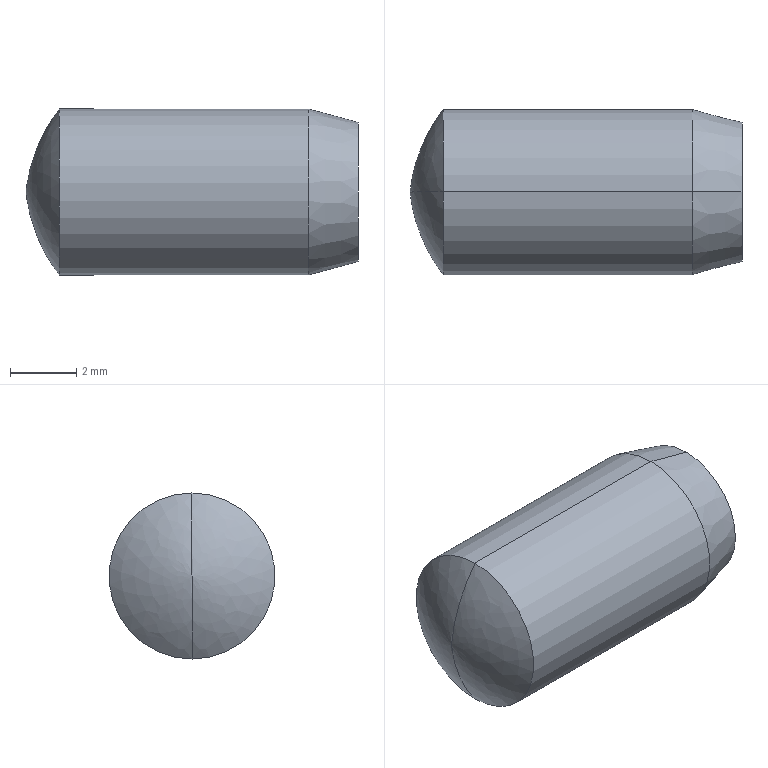Part | STEP file | 0243_009_MSC5-10 | 1 solid | 7 faces | box 10 x 5 x 5 mm | volume 181.449 mm3 | spline 2 | cylinder 2 | cone 2 | plane 1 | commonest cylinder face diameters 5 x2
STEP:
#1=CARTESIAN_POINT('',(0.,0.,0.));
#2=DIRECTION('',(0.,0.,1.));
#3=DIRECTION('',(1.,0.,0.));
#4=AXIS2_PLACEMENT_3D('',#1,#2,#3);
#5=CARTESIAN_POINT('',(-5.,0.,0.));
#6=VERTEX_POINT('',#5);
#7=CARTESIAN_POINT('',(-4.,0.,2.5));
#8=VERTEX_POINT('',#7);
#9=CARTESIAN_POINT('',(-0.02907,0.,-0.5384));
#10=DIRECTION('',(0.,1.,0.));
#11=DIRECTION('',(0.,0.,1.));
#12=AXIS2_PLACEMENT_3D('',#9,#10,#11);
#13=CIRCLE('',#12,5.);
#14=CARTESIAN_POINT('',(-5.,0.,0.));
#15=CARTESIAN_POINT('',(-5.,0.,0.));
#16=CARTESIAN_POINT('',(-5.,0.,0.));
#17=CARTESIAN_POINT('',(-5.,0.,0.));
#18=CARTESIAN_POINT('',(-4.901,0.,-0.9148));
#19=CARTESIAN_POINT('',(-4.901,-1.83,-0.9148));
#20=CARTESIAN_POINT('',(-4.901,-1.83,0.9148));
#21=CARTESIAN_POINT('',(-4.901,0.,0.9148));
#22=CARTESIAN_POINT('',(-4.559,0.,-1.769));
#23=CARTESIAN_POINT('',(-4.559,-3.538,-1.769));
#24=CARTESIAN_POINT('',(-4.559,-3.538,1.769));
#25=CARTESIAN_POINT('',(-4.559,0.,1.769));
#26=CARTESIAN_POINT('',(-4.,0.,-2.5));
#27=CARTESIAN_POINT('',(-4.,-5.,-2.5));
#28=CARTESIAN_POINT('',(-4.,-5.,2.5));
#29=CARTESIAN_POINT('',(-4.,0.,2.5));
#30=(BOUNDED_SURFACE()B_SPLINE_SURFACE(3,3,((#14,#15,#16,#17),(#18,#19,#20,#21),(#22,#23,#24,#25),(#26,#27,#28,#29)),.UNSPECIFIED.,.F.,.F.,.F.)B_SPLINE_SURFACE_WITH_KNOTS((4,4),(4,4),(0.,1.),(0.,1.),.PIECEWISE_BEZIER_KNOTS.)GEOMETRIC_REPRESENTATION_ITEM()RATIONAL_B_SPLINE_SURFACE(((1.,0.3333,0.3333,1.),(0.9754,0.3251,0.3251,0.9754),(0.9754,0.3251,0.3251,0.9754),(1.,0.3333,0.3333,1.)))REPRESENTATION_ITEM('')SURFACE());
#31=CARTESIAN_POINT('',(0.,1.));
#32=CARTESIAN_POINT('',(0.01534,1.));
#33=CARTESIAN_POINT('',(0.04597,1.));
#34=CARTESIAN_POINT('',(0.09177,1.));
#35=CARTESIAN_POINT('',(0.1374,1.));
#36=CARTESIAN_POINT('',(0.183,1.));
#37=CARTESIAN_POINT('',(0.2285,1.));
#38=CARTESIAN_POINT('',(0.2739,1.));
#39=CARTESIAN_POINT('',(0.3192,1.));
#40=CARTESIAN_POINT('',(0.3644,1.));
#41=CARTESIAN_POINT('',(0.4096,1.));
#42=CARTESIAN_POINT('',(0.4548,1.));
#43=CARTESIAN_POINT('',(0.5,1.));
#44=CARTESIAN_POINT('',(0.5452,1.));
#45=CARTESIAN_POINT('',(0.5904,1.));
#46=CARTESIAN_POINT('',(0.6356,1.));
#47=CARTESIAN_POINT('',(0.6808,1.));
#48=CARTESIAN_POINT('',(0.7261,1.));
#49=CARTESIAN_POINT('',(0.7715,1.));
#50=CARTESIAN_POINT('',(0.817,1.));
#51=CARTESIAN_POINT('',(0.8626,1.));
#52=CARTESIAN_POINT('',(0.9082,1.));
#53=CARTESIAN_POINT('',(0.954,1.));
#54=CARTESIAN_POINT('',(0.9847,1.));
#55=CARTESIAN_POINT('',(1.,1.));
#56=B_SPLINE_CURVE_WITH_KNOTS('',3,(#31,#32,#33,#34,#35,#36,#37,#38,#39,#40,#41,#42,#43,#44,#45,#46,#47,#48,#49,#50,#51,#52,#53,#54,#55),.UNSPECIFIED.,.F.,.F.,(4,1,1,1,1,1,1,1,1,1,1,1,1,1,1,1,1,1,1,1,1,1,4),(4.82,4.845,4.87,4.895,4.919,4.944,4.969,4.994,5.019,5.043,5.068,5.093,5.118,5.142,5.167,5.192,5.217,5.242,5.266,5.291,5.316,5.341,5.366),.QUASI_UNIFORM_KNOTS.);
#57=(GEOMETRIC_REPRESENTATION_CONTEXT(2)PARAMETRIC_REPRESENTATION_CONTEXT()REPRESENTATION_CONTEXT('',''));
#58=DEFINITIONAL_REPRESENTATION('',(#56),#57);
#59=PCURVE('',#30,#58);
#60=CARTESIAN_POINT('',(-5.,0.,0.));
#61=CARTESIAN_POINT('',(-5.,0.,0.));
#62=CARTESIAN_POINT('',(-5.,0.,0.));
#63=CARTESIAN_POINT('',(-5.,0.,0.));
#64=CARTESIAN_POINT('',(-4.901,0.,0.9148));
#65=CARTESIAN_POINT('',(-4.901,1.83,0.9148));
#66=CARTESIAN_POINT('',(-4.901,1.83,-0.9148));
#67=CARTESIAN_POINT('',(-4.901,0.,-0.9148));
#68=CARTESIAN_POINT('',(-4.559,0.,1.769));
#69=CARTESIAN_POINT('',(-4.559,3.538,1.769));
#70=CARTESIAN_POINT('',(-4.559,3.538,-1.769));
#71=CARTESIAN_POINT('',(-4.559,0.,-1.769));
#72=CARTESIAN_POINT('',(-4.,0.,2.5));
#73=CARTESIAN_POINT('',(-4.,5.,2.5));
#74=CARTESIAN_POINT('',(-4.,5.,-2.5));
#75=CARTESIAN_POINT('',(-4.,0.,-2.5));
#76=(BOUNDED_SURFACE()B_SPLINE_SURFACE(3,3,((#60,#61,#62,#63),(#64,#65,#66,#67),(#68,#69,#70,#71),(#72,#73,#74,#75)),.UNSPECIFIED.,.F.,.F.,.F.)B_SPLINE_SURFACE_WITH_KNOTS((4,4),(4,4),(0.,1.),(0.,1.),.PIECEWISE_BEZIER_KNOTS.)GEOMETRIC_REPRESENTATION_ITEM()RATIONAL_B_SPLINE_SURFACE(((1.,0.3333,0.3333,1.),(0.9754,0.3251,0.3251,0.9754),(0.9754,0.3251,0.3251,0.9754),(1.,0.3333,0.3333,1.)))REPRESENTATION_ITEM('')SURFACE());
#77=CARTESIAN_POINT('',(0.,0.));
#78=CARTESIAN_POINT('',(0.01534,0.));
#79=CARTESIAN_POINT('',(0.04597,0.));
#80=CARTESIAN_POINT('',(0.09177,0.));
#81=CARTESIAN_POINT('',(0.1374,0.));
#82=CARTESIAN_POINT('',(0.183,0.));
#83=CARTESIAN_POINT('',(0.2285,0.));
#84=CARTESIAN_POINT('',(0.2739,0.));
#85=CARTESIAN_POINT('',(0.3192,0.));
#86=CARTESIAN_POINT('',(0.3644,0.));
#87=CARTESIAN_POINT('',(0.4096,0.));
#88=CARTESIAN_POINT('',(0.4548,0.));
#89=CARTESIAN_POINT('',(0.5,0.));
#90=CARTESIAN_POINT('',(0.5452,0.));
#91=CARTESIAN_POINT('',(0.5904,0.));
#92=CARTESIAN_POINT('',(0.6356,0.));
#93=CARTESIAN_POINT('',(0.6808,0.));
#94=CARTESIAN_POINT('',(0.7261,0.));
#95=CARTESIAN_POINT('',(0.7715,0.));
#96=CARTESIAN_POINT('',(0.817,0.));
#97=CARTESIAN_POINT('',(0.8626,0.));
#98=CARTESIAN_POINT('',(0.9082,0.));
#99=CARTESIAN_POINT('',(0.954,0.));
#100=CARTESIAN_POINT('',(0.9847,0.));
#101=CARTESIAN_POINT('',(1.,0.));
#102=B_SPLINE_CURVE_WITH_KNOTS('',3,(#77,#78,#79,#80,#81,#82,#83,#84,#85,#86,#87,#88,#89,#90,#91,#92,#93,#94,#95,#96,#97,#98,#99,#100,#101),.UNSPECIFIED.,.F.,.F.,(4,1,1,1,1,1,1,1,1,1,1,1,1,1,1,1,1,1,1,1,1,1,4),(4.82,4.845,4.87,4.895,4.919,4.944,4.969,4.994,5.019,5.043,5.068,5.093,5.118,5.142,5.167,5.192,5.217,5.242,5.266,5.291,5.316,5.341,5.366),.QUASI_UNIFORM_KNOTS.);
#103=(GEOMETRIC_REPRESENTATION_CONTEXT(2)PARAMETRIC_REPRESENTATION_CONTEXT()REPRESENTATION_CONTEXT('',''));
#104=DEFINITIONAL_REPRESENTATION('',(#102),#103);
#105=PCURVE('',#76,#104);
#106=SURFACE_CURVE('',#13,(#59,#105),.PCURVE_S1.);
#107=EDGE_CURVE('',#6,#8,#106,.T.);
#108=ORIENTED_EDGE('',*,*,#107,.F.);
#109=CARTESIAN_POINT('',(-4.,0.,-2.5));
#110=VERTEX_POINT('',#109);
#111=CARTESIAN_POINT('',(-0.02907,0.,0.5384));
#112=DIRECTION('',(0.,-1.,0.));
#113=DIRECTION('',(0.,0.,-1.));
#114=AXIS2_PLACEMENT_3D('',#111,#112,#113);
#115=CIRCLE('',#114,5.);
#116=CARTESIAN_POINT('',(0.,0.));
#117=CARTESIAN_POINT('',(0.01534,0.));
#118=CARTESIAN_POINT('',(0.04597,0.));
#119=CARTESIAN_POINT('',(0.09177,0.));
#120=CARTESIAN_POINT('',(0.1374,0.));
#121=CARTESIAN_POINT('',(0.183,0.));
#122=CARTESIAN_POINT('',(0.2285,0.));
#123=CARTESIAN_POINT('',(0.2739,0.));
#124=CARTESIAN_POINT('',(0.3192,0.));
#125=CARTESIAN_POINT('',(0.3644,0.));
#126=CARTESIAN_POINT('',(0.4096,0.));
#127=CARTESIAN_POINT('',(0.4548,0.));
#128=CARTESIAN_POINT('',(0.5,0.));
#129=CARTESIAN_POINT('',(0.5452,0.));
#130=CARTESIAN_POINT('',(0.5904,0.));
#131=CARTESIAN_POINT('',(0.6356,0.));
#132=CARTESIAN_POINT('',(0.6808,0.));
#133=CARTESIAN_POINT('',(0.7261,0.));
#134=CARTESIAN_POINT('',(0.7715,0.));
#135=CARTESIAN_POINT('',(0.817,0.));
#136=CARTESIAN_POINT('',(0.8626,0.));
#137=CARTESIAN_POINT('',(0.9082,0.));
#138=CARTESIAN_POINT('',(0.954,0.));
#139=CARTESIAN_POINT('',(0.9847,0.));
#140=CARTESIAN_POINT('',(1.,0.));
#141=B_SPLINE_CURVE_WITH_KNOTS('',3,(#116,#117,#118,#119,#120,#121,#122,#123,#124,#125,#126,#127,#128,#129,#130,#131,#132,#133,#134,#135,#136,#137,#138,#139,#140),.UNSPECIFIED.,.F.,.F.,(4,1,1,1,1,1,1,1,1,1,1,1,1,1,1,1,1,1,1,1,1,1,4),(4.82,4.845,4.87,4.895,4.919,4.944,4.969,4.994,5.019,5.043,5.068,5.093,5.118,5.142,5.167,5.192,5.217,5.242,5.266,5.291,5.316,5.341,5.366),.QUASI_UNIFORM_KNOTS.);
#142=(GEOMETRIC_REPRESENTATION_CONTEXT(2)PARAMETRIC_REPRESENTATION_CONTEXT()REPRESENTATION_CONTEXT('',''));
#143=DEFINITIONAL_REPRESENTATION('',(#141),#142);
#144=PCURVE('',#30,#143);
#145=CARTESIAN_POINT('',(0.,1.));
#146=CARTESIAN_POINT('',(0.01534,1.));
#147=CARTESIAN_POINT('',(0.04597,1.));
#148=CARTESIAN_POINT('',(0.09177,1.));
#149=CARTESIAN_POINT('',(0.1374,1.));
#150=CARTESIAN_POINT('',(0.183,1.));
#151=CARTESIAN_POINT('',(0.2285,1.));
#152=CARTESIAN_POINT('',(0.2739,1.));
#153=CARTESIAN_POINT('',(0.3192,1.));
#154=CARTESIAN_POINT('',(0.3644,1.));
#155=CARTESIAN_POINT('',(0.4096,1.));
#156=CARTESIAN_POINT('',(0.4548,1.));
#157=CARTESIAN_POINT('',(0.5,1.));
#158=CARTESIAN_POINT('',(0.5452,1.));
#159=CARTESIAN_POINT('',(0.5904,1.));
#160=CARTESIAN_POINT('',(0.6356,1.));
#161=CARTESIAN_POINT('',(0.6808,1.));
#162=CARTESIAN_POINT('',(0.7261,1.));
#163=CARTESIAN_POINT('',(0.7715,1.));
#164=CARTESIAN_POINT('',(0.817,1.));
#165=CARTESIAN_POINT('',(0.8626,1.));
#166=CARTESIAN_POINT('',(0.9082,1.));
#167=CARTESIAN_POINT('',(0.954,1.));
#168=CARTESIAN_POINT('',(0.9847,1.));
#169=CARTESIAN_POINT('',(1.,1.));
#170=B_SPLINE_CURVE_WITH_KNOTS('',3,(#145,#146,#147,#148,#149,#150,#151,#152,#153,#154,#155,#156,#157,#158,#159,#160,#161,#162,#163,#164,#165,#166,#167,#168,#169),.UNSPECIFIED.,.F.,.F.,(4,1,1,1,1,1,1,1,1,1,1,1,1,1,1,1,1,1,1,1,1,1,4),(4.82,4.845,4.87,4.895,4.919,4.944,4.969,4.994,5.019,5.043,5.068,5.093,5.118,5.142,5.167,5.192,5.217,5.242,5.266,5.291,5.316,5.341,5.366),.QUASI_UNIFORM_KNOTS.);
#171=(GEOMETRIC_REPRESENTATION_CONTEXT(2)PARAMETRIC_REPRESENTATION_CONTEXT()REPRESENTATION_CONTEXT('',''));
#172=DEFINITIONAL_REPRESENTATION('',(#170),#171);
#173=PCURVE('',#76,#172);
#174=SURFACE_CURVE('',#115,(#144,#173),.PCURVE_S1.);
#175=EDGE_CURVE('',#6,#110,#174,.T.);
#176=ORIENTED_EDGE('',*,*,#175,.T.);
#177=CARTESIAN_POINT('',(-4.,0.,0.));
#178=DIRECTION('',(1.,0.,0.));
#179=DIRECTION('',(0.,0.,-1.));
#180=AXIS2_PLACEMENT_3D('',#177,#178,#179);
#181=CIRCLE('',#180,2.5);
#182=CARTESIAN_POINT('',(1.,1.));
#183=CARTESIAN_POINT('',(1.,0.9763));
#184=CARTESIAN_POINT('',(1.,0.9319));
#185=CARTESIAN_POINT('',(1.,0.8733));
#186=CARTESIAN_POINT('',(1.,0.8206));
#187=CARTESIAN_POINT('',(1.,0.7724));
#188=CARTESIAN_POINT('',(1.,0.7279));
#189=CARTESIAN_POINT('',(1.,0.6861));
#190=CARTESIAN_POINT('',(1.,0.6465));
#191=CARTESIAN_POINT('',(1.,0.6086));
#192=CARTESIAN_POINT('',(1.,0.5718));
#193=CARTESIAN_POINT('',(1.,0.5357));
#194=CARTESIAN_POINT('',(1.,0.5));
#195=CARTESIAN_POINT('',(1.,0.4643));
#196=CARTESIAN_POINT('',(1.,0.4282));
#197=CARTESIAN_POINT('',(1.,0.3914));
#198=CARTESIAN_POINT('',(1.,0.3535));
#199=CARTESIAN_POINT('',(1.,0.3139));
#200=CARTESIAN_POINT('',(1.,0.2721));
#201=CARTESIAN_POINT('',(1.,0.2276));
#202=CARTESIAN_POINT('',(1.,0.1794));
#203=CARTESIAN_POINT('',(1.,0.1267));
#204=CARTESIAN_POINT('',(1.,0.06805));
#205=CARTESIAN_POINT('',(1.,0.02375));
#206=CARTESIAN_POINT('',(1.,0.));
#207=B_SPLINE_CURVE_WITH_KNOTS('',3,(#182,#183,#184,#185,#186,#187,#188,#189,#190,#191,#192,#193,#194,#195,#196,#197,#198,#199,#200,#201,#202,#203,#204,#205,#206),.UNSPECIFIED.,.F.,.F.,(4,1,1,1,1,1,1,1,1,1,1,1,1,1,1,1,1,1,1,1,1,1,4),(3.142,3.284,3.427,3.57,3.713,3.856,3.998,4.141,4.284,4.427,4.57,4.712,4.855,4.998,5.141,5.284,5.426,5.569,5.712,5.855,5.998,6.14,6.283),.QUASI_UNIFORM_KNOTS.);
#208=(GEOMETRIC_REPRESENTATION_CONTEXT(2)PARAMETRIC_REPRESENTATION_CONTEXT()REPRESENTATION_CONTEXT('',''));
#209=DEFINITIONAL_REPRESENTATION('',(#207),#208);
#210=PCURVE('',#30,#209);
#211=CARTESIAN_POINT('',(-0.25,0.,0.));
#212=DIRECTION('',(1.,0.,0.));
#213=DIRECTION('',(0.,0.,-1.));
#214=AXIS2_PLACEMENT_3D('',#211,#212,#213);
#215=CYLINDRICAL_SURFACE('',#214,2.5);
#216=CARTESIAN_POINT('',(0.,-3.75));
#217=DIRECTION('',(1.,0.));
#218=VECTOR('',#217,1.);
#219=LINE('',#216,#218);
#220=(GEOMETRIC_REPRESENTATION_CONTEXT(2)PARAMETRIC_REPRESENTATION_CONTEXT()REPRESENTATION_CONTEXT('',''));
#221=DEFINITIONAL_REPRESENTATION('',(#219),#220);
#222=PCURVE('',#215,#221);
#223=SURFACE_CURVE('',#181,(#210,#222),.PCURVE_S1.);
#224=EDGE_CURVE('',#8,#110,#223,.T.);
#225=ORIENTED_EDGE('',*,*,#224,.F.);
#226=EDGE_LOOP('',(#108,#176,#225));
#227=FACE_BOUND('',#226,.T.);
#228=ADVANCED_FACE('',(#227),#30,.T.);
#229=CARTESIAN_POINT('',(-4.,0.,0.));
#230=DIRECTION('',(1.,0.,0.));
#231=DIRECTION('',(0.,0.,-1.));
#232=AXIS2_PLACEMENT_3D('',#229,#230,#231);
#233=CIRCLE('',#232,2.5);
#234=CARTESIAN_POINT('',(-0.25,0.,0.));
#235=DIRECTION('',(1.,0.,0.));
#236=DIRECTION('',(0.,0.,-1.));
#237=AXIS2_PLACEMENT_3D('',#234,#235,#236);
#238=CYLINDRICAL_SURFACE('',#237,2.5);
#239=CARTESIAN_POINT('',(0.,-3.75));
#240=DIRECTION('',(1.,0.));
#241=VECTOR('',#240,1.);
#242=LINE('',#239,#241);
#243=(GEOMETRIC_REPRESENTATION_CONTEXT(2)PARAMETRIC_REPRESENTATION_CONTEXT()REPRESENTATION_CONTEXT('',''));
#244=DEFINITIONAL_REPRESENTATION('',(#242),#243);
#245=PCURVE('',#238,#244);
#246=CARTESIAN_POINT('',(1.,1.));
#247=CARTESIAN_POINT('',(1.,0.9763));
#248=CARTESIAN_POINT('',(1.,0.9319));
#249=CARTESIAN_POINT('',(1.,0.8733));
#250=CARTESIAN_POINT('',(1.,0.8206));
#251=CARTESIAN_POINT('',(1.,0.7724));
#252=CARTESIAN_POINT('',(1.,0.7279));
#253=CARTESIAN_POINT('',(1.,0.6861));
#254=CARTESIAN_POINT('',(1.,0.6465));
#255=CARTESIAN_POINT('',(1.,0.6086));
#256=CARTESIAN_POINT('',(1.,0.5718));
#257=CARTESIAN_POINT('',(1.,0.5357));
#258=CARTESIAN_POINT('',(1.,0.5));
#259=CARTESIAN_POINT('',(1.,0.4643));
#260=CARTESIAN_POINT('',(1.,0.4282));
#261=CARTESIAN_POINT('',(1.,0.3914));
#262=CARTESIAN_POINT('',(1.,0.3535));
#263=CARTESIAN_POINT('',(1.,0.3139));
#264=CARTESIAN_POINT('',(1.,0.2721));
#265=CARTESIAN_POINT('',(1.,0.2276));
#266=CARTESIAN_POINT('',(1.,0.1794));
#267=CARTESIAN_POINT('',(1.,0.1267));
#268=CARTESIAN_POINT('',(1.,0.06805));
#269=CARTESIAN_POINT('',(1.,0.02375));
#270=CARTESIAN_POINT('',(1.,0.));
#271=B_SPLINE_CURVE_WITH_KNOTS('',3,(#246,#247,#248,#249,#250,#251,#252,#253,#254,#255,#256,#257,#258,#259,#260,#261,#262,#263,#264,#265,#266,#267,#268,#269,#270),.UNSPECIFIED.,.F.,.F.,(4,1,1,1,1,1,1,1,1,1,1,1,1,1,1,1,1,1,1,1,1,1,4),(0.,0.1428,0.2856,0.4284,0.5712,0.714,0.8568,0.9996,1.142,1.285,1.428,1.571,1.714,1.856,1.999,2.142,2.285,2.428,2.57,2.713,2.856,2.999,3.142),.QUASI_UNIFORM_KNOTS.);
#272=(GEOMETRIC_REPRESENTATION_CONTEXT(2)PARAMETRIC_REPRESENTATION_CONTEXT()REPRESENTATION_CONTEXT('',''));
#273=DEFINITIONAL_REPRESENTATION('',(#271),#272);
#274=PCURVE('',#76,#273);
#275=SURFACE_CURVE('',#233,(#245,#274),.PCURVE_S1.);
#276=EDGE_CURVE('',#110,#8,#275,.T.);
#277=ORIENTED_EDGE('',*,*,#276,.T.);
#278=CARTESIAN_POINT('',(3.5,0.,2.5));
#279=VERTEX_POINT('',#278);
#280=CARTESIAN_POINT('',(-0.25,0.,2.5));
#281=DIRECTION('',(1.,0.,0.));
#282=VECTOR('',#281,1.);
#283=LINE('',#280,#282);
#284=CARTESIAN_POINT('',(3.142,0.));
#285=DIRECTION('',(0.,1.));
#286=VECTOR('',#285,1.);
#287=LINE('',#284,#286);
#288=(GEOMETRIC_REPRESENTATION_CONTEXT(2)PARAMETRIC_REPRESENTATION_CONTEXT()REPRESENTATION_CONTEXT('',''));
#289=DEFINITIONAL_REPRESENTATION('',(#287),#288);
#290=PCURVE('',#238,#289);
#291=CARTESIAN_POINT('',(3.142,0.));
#292=DIRECTION('',(0.,1.));
#293=VECTOR('',#292,1.);
#294=LINE('',#291,#293);
#295=(GEOMETRIC_REPRESENTATION_CONTEXT(2)PARAMETRIC_REPRESENTATION_CONTEXT()REPRESENTATION_CONTEXT('',''));
#296=DEFINITIONAL_REPRESENTATION('',(#294),#295);
#297=PCURVE('',#215,#296);
#298=SURFACE_CURVE('',#283,(#290,#297),.PCURVE_S1.);
#299=EDGE_CURVE('',#8,#279,#298,.T.);
#300=ORIENTED_EDGE('',*,*,#299,.T.);
#301=CARTESIAN_POINT('',(3.5,0.,-2.5));
#302=VERTEX_POINT('',#301);
#303=CARTESIAN_POINT('',(3.5,0.,0.));
#304=DIRECTION('',(-1.,0.,0.));
#305=DIRECTION('',(0.,0.,-1.));
#306=AXIS2_PLACEMENT_3D('',#303,#304,#305);
#307=CIRCLE('',#306,2.5);
#308=CARTESIAN_POINT('',(6.283,3.75));
#309=DIRECTION('',(-1.,0.));
#310=VECTOR('',#309,1.);
#311=LINE('',#308,#310);
#312=(GEOMETRIC_REPRESENTATION_CONTEXT(2)PARAMETRIC_REPRESENTATION_CONTEXT()REPRESENTATION_CONTEXT('',''));
#313=DEFINITIONAL_REPRESENTATION('',(#311),#312);
#314=PCURVE('',#238,#313);
#315=CARTESIAN_POINT('',(3.5,0.,0.));
#316=DIRECTION('',(-1.,0.,0.));
#317=DIRECTION('',(0.,0.,1.));
#318=AXIS2_PLACEMENT_3D('',#315,#316,#317);
#319=CONICAL_SURFACE('',#318,2.5,0.2618);
#320=CARTESIAN_POINT('',(-3.142,0.));
#321=DIRECTION('',(1.,0.));
#322=VECTOR('',#321,1.);
#323=LINE('',#320,#322);
#324=(GEOMETRIC_REPRESENTATION_CONTEXT(2)PARAMETRIC_REPRESENTATION_CONTEXT()REPRESENTATION_CONTEXT('',''));
#325=DEFINITIONAL_REPRESENTATION('',(#323),#324);
#326=PCURVE('',#319,#325);
#327=SURFACE_CURVE('',#307,(#314,#326),.PCURVE_S1.);
#328=EDGE_CURVE('',#279,#302,#327,.T.);
#329=ORIENTED_EDGE('',*,*,#328,.T.);
#330=CARTESIAN_POINT('',(-0.25,0.,-2.5));
#331=DIRECTION('',(1.,0.,0.));
#332=VECTOR('',#331,1.);
#333=LINE('',#330,#332);
#334=CARTESIAN_POINT('',(0.,0.));
#335=DIRECTION('',(0.,1.));
#336=VECTOR('',#335,1.);
#337=LINE('',#334,#336);
#338=(GEOMETRIC_REPRESENTATION_CONTEXT(2)PARAMETRIC_REPRESENTATION_CONTEXT()REPRESENTATION_CONTEXT('',''));
#339=DEFINITIONAL_REPRESENTATION('',(#337),#338);
#340=PCURVE('',#238,#339);
#341=CARTESIAN_POINT('',(6.283,0.));
#342=DIRECTION('',(0.,1.));
#343=VECTOR('',#342,1.);
#344=LINE('',#341,#343);
#345=(GEOMETRIC_REPRESENTATION_CONTEXT(2)PARAMETRIC_REPRESENTATION_CONTEXT()REPRESENTATION_CONTEXT('',''));
#346=DEFINITIONAL_REPRESENTATION('',(#344),#345);
#347=PCURVE('',#215,#346);
#348=SURFACE_CURVE('',#333,(#340,#347),.PCURVE_S1.);
#349=EDGE_CURVE('',#110,#302,#348,.T.);
#350=ORIENTED_EDGE('',*,*,#349,.F.);
#351=EDGE_LOOP('',(#277,#300,#329,#350));
#352=FACE_BOUND('',#351,.T.);
#353=ADVANCED_FACE('',(#352),#238,.T.);
#354=CARTESIAN_POINT('',(5.,0.,2.098));
#355=VERTEX_POINT('',#354);
#356=CARTESIAN_POINT('',(5.,0.,-2.098));
#357=VERTEX_POINT('',#356);
#358=CARTESIAN_POINT('',(5.,0.,0.));
#359=DIRECTION('',(-1.,0.,0.));
#360=DIRECTION('',(0.,0.,1.));
#361=AXIS2_PLACEMENT_3D('',#358,#359,#360);
#362=CIRCLE('',#361,2.098);
#363=CARTESIAN_POINT('',(0.,-1.5));
#364=DIRECTION('',(1.,0.));
#365=VECTOR('',#364,1.);
#366=LINE('',#363,#365);
#367=(GEOMETRIC_REPRESENTATION_CONTEXT(2)PARAMETRIC_REPRESENTATION_CONTEXT()REPRESENTATION_CONTEXT('',''));
#368=DEFINITIONAL_REPRESENTATION('',(#366),#367);
#369=PCURVE('',#319,#368);
#370=CARTESIAN_POINT('',(5.,1.049,0.));
#371=DIRECTION('',(1.,0.,0.));
#372=DIRECTION('',(0.,0.,-1.));
#373=AXIS2_PLACEMENT_3D('',#370,#371,#372);
#374=PLANE('',#373);
#375=CARTESIAN_POINT('',(-2.098,-1.049));
#376=CARTESIAN_POINT('',(-2.098,2.585));
#377=CARTESIAN_POINT('',(1.049,0.7679));
#378=CARTESIAN_POINT('',(4.196,-1.049));
#379=CARTESIAN_POINT('',(1.049,-2.866));
#380=CARTESIAN_POINT('',(-2.098,-4.683));
#381=CARTESIAN_POINT('',(-2.098,-1.049));
#382=(BOUNDED_CURVE()B_SPLINE_CURVE(2,(#375,#376,#377,#378,#379,#380,#381),.UNSPECIFIED.,.T.,.F.)B_SPLINE_CURVE_WITH_KNOTS((1,2,2,2,2,1),(-2.094,0.,2.094,4.189,6.283,8.378),.UNSPECIFIED.)CURVE()GEOMETRIC_REPRESENTATION_ITEM()RATIONAL_B_SPLINE_CURVE((1.,0.5,1.,0.5,1.,0.5,1.))REPRESENTATION_ITEM(''));
#383=(GEOMETRIC_REPRESENTATION_CONTEXT(2)PARAMETRIC_REPRESENTATION_CONTEXT()REPRESENTATION_CONTEXT('',''));
#384=DEFINITIONAL_REPRESENTATION('',(#382),#383);
#385=PCURVE('',#374,#384);
#386=SURFACE_CURVE('',#362,(#369,#385),.PCURVE_S1.);
#387=EDGE_CURVE('',#355,#357,#386,.T.);
#388=ORIENTED_EDGE('',*,*,#387,.T.);
#389=CARTESIAN_POINT('',(3.5,0.,-2.5));
#390=DIRECTION('',(-0.9659,0.,-0.2588));
#391=VECTOR('',#390,1.);
#392=LINE('',#389,#391);
#393=CARTESIAN_POINT('',(3.142,0.));
#394=DIRECTION('',(0.,1.));
#395=VECTOR('',#394,1.);
#396=LINE('',#393,#395);
#397=(GEOMETRIC_REPRESENTATION_CONTEXT(2)PARAMETRIC_REPRESENTATION_CONTEXT()REPRESENTATION_CONTEXT('',''));
#398=DEFINITIONAL_REPRESENTATION('',(#396),#397);
#399=PCURVE('',#319,#398);
#400=CARTESIAN_POINT('',(3.5,0.,0.));
#401=DIRECTION('',(-1.,0.,0.));
#402=DIRECTION('',(0.,0.,1.));
#403=AXIS2_PLACEMENT_3D('',#400,#401,#402);
#404=CONICAL_SURFACE('',#403,2.5,0.2618);
#405=CARTESIAN_POINT('',(3.142,0.));
#406=DIRECTION('',(0.,1.));
#407=VECTOR('',#406,1.);
#408=LINE('',#405,#407);
#409=(GEOMETRIC_REPRESENTATION_CONTEXT(2)PARAMETRIC_REPRESENTATION_CONTEXT()REPRESENTATION_CONTEXT('',''));
#410=DEFINITIONAL_REPRESENTATION('',(#408),#409);
#411=PCURVE('',#404,#410);
#412=SURFACE_CURVE('',#392,(#399,#411),.PCURVE_S1.);
#413=EDGE_CURVE('',#357,#302,#412,.T.);
#414=ORIENTED_EDGE('',*,*,#413,.T.);
#415=ORIENTED_EDGE('',*,*,#328,.F.);
#416=CARTESIAN_POINT('',(3.5,0.,2.5));
#417=DIRECTION('',(-0.9659,0.,0.2588));
#418=VECTOR('',#417,1.);
#419=LINE('',#416,#418);
#420=CARTESIAN_POINT('',(0.,0.));
#421=DIRECTION('',(0.,1.));
#422=VECTOR('',#421,1.);
#423=LINE('',#420,#422);
#424=(GEOMETRIC_REPRESENTATION_CONTEXT(2)PARAMETRIC_REPRESENTATION_CONTEXT()REPRESENTATION_CONTEXT('',''));
#425=DEFINITIONAL_REPRESENTATION('',(#423),#424);
#426=PCURVE('',#319,#425);
#427=CARTESIAN_POINT('',(6.283,0.));
#428=DIRECTION('',(0.,1.));
#429=VECTOR('',#428,1.);
#430=LINE('',#427,#429);
#431=(GEOMETRIC_REPRESENTATION_CONTEXT(2)PARAMETRIC_REPRESENTATION_CONTEXT()REPRESENTATION_CONTEXT('',''));
#432=DEFINITIONAL_REPRESENTATION('',(#430),#431);
#433=PCURVE('',#404,#432);
#434=SURFACE_CURVE('',#419,(#426,#433),.PCURVE_S1.);
#435=EDGE_CURVE('',#355,#279,#434,.T.);
#436=ORIENTED_EDGE('',*,*,#435,.F.);
#437=EDGE_LOOP('',(#388,#414,#415,#436));
#438=FACE_BOUND('',#437,.T.);
#439=ADVANCED_FACE('',(#438),#319,.T.);
#440=ORIENTED_EDGE('',*,*,#299,.F.);
#441=ORIENTED_EDGE('',*,*,#224,.T.);
#442=ORIENTED_EDGE('',*,*,#349,.T.);
#443=CARTESIAN_POINT('',(3.5,0.,0.));
#444=DIRECTION('',(-1.,0.,0.));
#445=DIRECTION('',(0.,0.,-1.));
#446=AXIS2_PLACEMENT_3D('',#443,#444,#445);
#447=CIRCLE('',#446,2.5);
#448=CARTESIAN_POINT('',(6.283,3.75));
#449=DIRECTION('',(-1.,0.));
#450=VECTOR('',#449,1.);
#451=LINE('',#448,#450);
#452=(GEOMETRIC_REPRESENTATION_CONTEXT(2)PARAMETRIC_REPRESENTATION_CONTEXT()REPRESENTATION_CONTEXT('',''));
#453=DEFINITIONAL_REPRESENTATION('',(#451),#452);
#454=PCURVE('',#215,#453);
#455=CARTESIAN_POINT('',(3.142,0.));
#456=DIRECTION('',(1.,0.));
#457=VECTOR('',#456,1.);
#458=LINE('',#455,#457);
#459=(GEOMETRIC_REPRESENTATION_CONTEXT(2)PARAMETRIC_REPRESENTATION_CONTEXT()REPRESENTATION_CONTEXT('',''));
#460=DEFINITIONAL_REPRESENTATION('',(#458),#459);
#461=PCURVE('',#404,#460);
#462=SURFACE_CURVE('',#447,(#454,#461),.PCURVE_S1.);
#463=EDGE_CURVE('',#302,#279,#462,.T.);
#464=ORIENTED_EDGE('',*,*,#463,.T.);
#465=EDGE_LOOP('',(#440,#441,#442,#464));
#466=FACE_BOUND('',#465,.T.);
#467=ADVANCED_FACE('',(#466),#215,.T.);
#468=ORIENTED_EDGE('',*,*,#175,.F.);
#469=ORIENTED_EDGE('',*,*,#107,.T.);
#470=ORIENTED_EDGE('',*,*,#276,.F.);
#471=EDGE_LOOP('',(#468,#469,#470));
#472=FACE_BOUND('',#471,.T.);
#473=ADVANCED_FACE('',(#472),#76,.T.);
#474=ORIENTED_EDGE('',*,*,#413,.F.);
#475=CARTESIAN_POINT('',(5.,0.,0.));
#476=DIRECTION('',(-1.,0.,0.));
#477=DIRECTION('',(0.,0.,1.));
#478=AXIS2_PLACEMENT_3D('',#475,#476,#477);
#479=CIRCLE('',#478,2.098);
#480=CARTESIAN_POINT('',(0.,-1.5));
#481=DIRECTION('',(1.,0.));
#482=VECTOR('',#481,1.);
#483=LINE('',#480,#482);
#484=(GEOMETRIC_REPRESENTATION_CONTEXT(2)PARAMETRIC_REPRESENTATION_CONTEXT()REPRESENTATION_CONTEXT('',''));
#485=DEFINITIONAL_REPRESENTATION('',(#483),#484);
#486=PCURVE('',#404,#485);
#487=CARTESIAN_POINT('',(-2.098,-1.049));
#488=CARTESIAN_POINT('',(-2.098,2.585));
#489=CARTESIAN_POINT('',(1.049,0.7679));
#490=CARTESIAN_POINT('',(4.196,-1.049));
#491=CARTESIAN_POINT('',(1.049,-2.866));
#492=CARTESIAN_POINT('',(-2.098,-4.683));
#493=CARTESIAN_POINT('',(-2.098,-1.049));
#494=(BOUNDED_CURVE()B_SPLINE_CURVE(2,(#487,#488,#489,#490,#491,#492,#493),.UNSPECIFIED.,.T.,.F.)B_SPLINE_CURVE_WITH_KNOTS((1,2,2,2,2,1),(-2.094,0.,2.094,4.189,6.283,8.378),.UNSPECIFIED.)CURVE()GEOMETRIC_REPRESENTATION_ITEM()RATIONAL_B_SPLINE_CURVE((1.,0.5,1.,0.5,1.,0.5,1.))REPRESENTATION_ITEM(''));
#495=(GEOMETRIC_REPRESENTATION_CONTEXT(2)PARAMETRIC_REPRESENTATION_CONTEXT()REPRESENTATION_CONTEXT('',''));
#496=DEFINITIONAL_REPRESENTATION('',(#494),#495);
#497=PCURVE('',#374,#496);
#498=SURFACE_CURVE('',#479,(#486,#497),.PCURVE_S1.);
#499=EDGE_CURVE('',#357,#355,#498,.T.);
#500=ORIENTED_EDGE('',*,*,#499,.T.);
#501=ORIENTED_EDGE('',*,*,#435,.T.);
#502=ORIENTED_EDGE('',*,*,#463,.F.);
#503=EDGE_LOOP('',(#474,#500,#501,#502));
#504=FACE_BOUND('',#503,.T.);
#505=ADVANCED_FACE('',(#504),#404,.T.);
#506=ORIENTED_EDGE('',*,*,#387,.F.);
#507=ORIENTED_EDGE('',*,*,#499,.F.);
#508=EDGE_LOOP('',(#506,#507));
#509=FACE_BOUND('',#508,.T.);
#510=ADVANCED_FACE('',(#509),#374,.T.);
#511=CLOSED_SHELL('',(#228,#353,#439,#467,#473,#505,#510));
#512=MANIFOLD_SOLID_BREP('',#511);
#513=(LENGTH_UNIT()NAMED_UNIT(*)SI_UNIT(.MILLI.,.METRE.));
#514=UNCERTAINTY_MEASURE_WITH_UNIT(LENGTH_MEASURE(0.0000001),#513,'','');
#515=(NAMED_UNIT(*)PLANE_ANGLE_UNIT()SI_UNIT($,.RADIAN.));
#516=(NAMED_UNIT(*)SI_UNIT($,.STERADIAN.)SOLID_ANGLE_UNIT());
#517=(GEOMETRIC_REPRESENTATION_CONTEXT(3)GLOBAL_UNCERTAINTY_ASSIGNED_CONTEXT((#514))GLOBAL_UNIT_ASSIGNED_CONTEXT((#513,#515,#516))REPRESENTATION_CONTEXT('',''));
#518=ADVANCED_BREP_SHAPE_REPRESENTATION('',(#4,#512),#517);